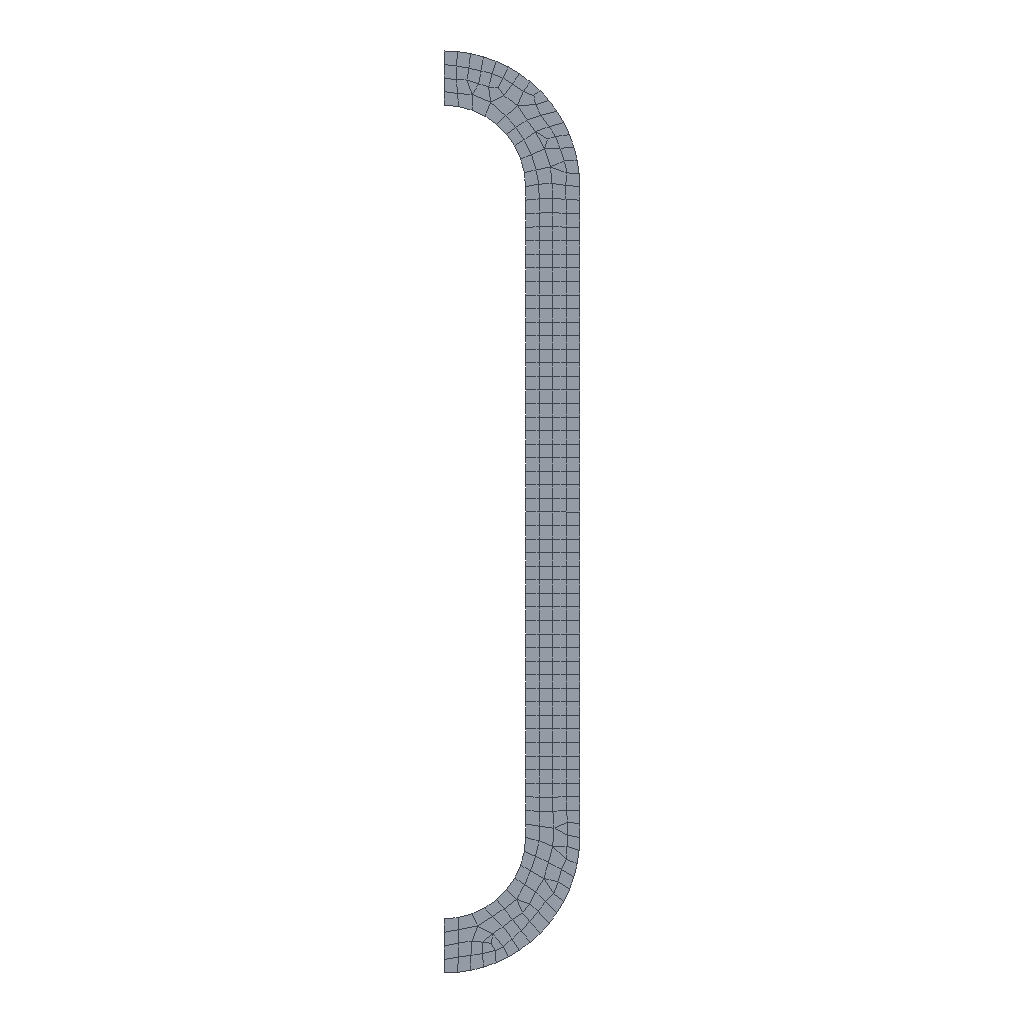Simulation study | ansys workbench
Set-up summary:
category,name,step,type,value,unit,region
solver,ansys_workbench
units,mm-N-s-tonne (MPa),,stated,"/units,MPA"
analysis,LS1,,static
load_step,LS1,LS1,static,nsubst=1; time=1
mesh,nodes,,,1039
mesh,elements,,,371
element_type,PLANE183,,,297
element_type,SURF153,,,66
element_type,CONTA172,,,8
material,?,,E,210000,tonne s^-2 mm^-1
material,?,,nu,0.3
material,?,,density,7.85e-09,tonne mm^-3
load,Define Pressure Using Surface Effect Elements,LS1,pressure,150,,SURF153 #4
bc,,LS1,fixed,"[dofs=UX,UY n=2]",,node list
contact,contact 1,,bonded (always),element=CONTA172
named_set,REMOTEDISPALL,,node,1
Ansys APDL input file, long lists of numbers shortened:
/batch
/config,noeldb,1     ! force off writing results to database
*get,_wallstrt,active,,time,wall
! ANSYS input file written by Workbench version 2021 R1
! File used for geometry attach:
/title,________--____ (A5)
! ****** Begin Custom Load Command Snippet ******
/COM, ACT Extensions:
/COM,     LSDYNA, 2021.1
/COM,
! ****** End   Custom Load Command Snippet ******
*DIM,_wb_ProjectScratch_dir,string,248
_wb_ProjectScratch_dir(1) = ''
*DIM,_wb_SolverFiles_dir,string,248
_wb_SolverFiles_dir(1) = ''
*DIM,_wb_userfiles_dir,string,248
_wb_userfiles_dir(1) = ''
/com,--- Data in consistent NMM units. See Solving Units in the help system for more information.
/units,MPA
/nopr
/wb,file,start              !  signify a WB generated input file
/prep7
! Turn off shape checking because checks already performed inside WB mesher.
! See help system for more information.
SHPP,OFF,,NOWARN
/nolist
etcon,set             ! allow ANSYS to choose best KEYOP's for 180x elements, resets any applicable keyopt to MAPDL defaults
/com,*********** Nodes for the whole assembly ***********
nblock,3,,1141
(1i9,3e20.9e3)
        1     0.000000000E+00     0.000000000E+00     0.000000000E+00
! (1037 more lines like these left out)
-1
/com,*********** Nodes for all Remote Points ***********
nblock,3
(1i9,3e20.9e3)
     1039     3.516693785E+01     1.699999993E+02     0.000000000E+00
-1
/wb,elem,start            !  set before creation of elements
/com,*********** Elements for Body 1 "______2-FreeParts|NONE" ***********
et,1,183
keyo,1,3,1
eblock,19,solid,,297
(19i9)
        1        1        1        1        0        0        0        0        8        0        1      158      197      195      195      688      826      195      687
! (296 more lines like these left out)
-1
/wb,elem,end               !  done creating elements
/com,*********** Send User Defined Coordinate System(s) ***********
csys,0
toffst,273.15,  ! Temperature offset from absolute zero
/com,*********** Set Reference Temperature ***********
tref,22.
/wb,mat,start              !  starting to send materials
/com,*********** Send Materials ***********
MP,DENS,1,7.85e-09,	! tonne mm^-3
MP,EX,1,210000,	! tonne s^-2 mm^-1
MP,NUXY,1,0.3,
/wb,mat,end                !  done sending materials
/com,*********** Send Sheet Properties ***********
!************************* Model Summary ********************
!______2-FreeParts|NONE,	合金钢,	matid,	1
!************************* End Model Summary ********************
! get the diagonal of the bounding box. Needed later for other things
*get,_xmin,node,,mnloc,x
*get,_ymin,node,,mnloc,y
*get,_zmin,node,,mnloc,z
*get,_xmax,node,,mxloc,x
*get,_ymax,node,,mxloc,y
*get,_zmax,node,,mxloc,z
_ASMDIAG=(_xmax-_xmin)*(_xmax-_xmin)+(_ymax-_ymin)*(_ymax-_ymin)+(_zmax-_zmin)*(_zmax-_zmin)
_ASMDIAG=SQRT(_ASMDIAG)
/wb,contact,start          !  starting to send contact
/wb,contact,end            !  done creating contacts
/golist
/wb,load,start             !  starting to send loads
/com,*********** Create Remote Point "内部远程点" ***********
! -------- Remote Point Used by "远程位移" --------
*set,tid,3
*set,cid,2
et,cid,172
et,tid,169
keyo,tid,2,1               ! Don't fix the pilot node
keyo,tid,4,000111
keyo,cid,12,5              ! Bonded Contact
keyo,cid,4,1               ! Deformable RBE3 style load
keyo,cid,2,2               ! MPC style contact
eblock,10,,,8
(15i9)
      299        2        2        2        0       84       85      537
! (7 more lines like these left out)
-1
*set,_npilot,1039
_npilot71=_npilot
type,tid
mat ,cid
real,cid
tshape,pilo
en,307,_npilot
tshape
/com,*********** Define Pressure Using Surface Effect Elements ***********
et,4,153
keyop,4,3,10        ! get plane stress option and thickness from underlying element
eblock,10,,,66
(15i9)
      308        4        4        4        0      143      151      654
! (65 more lines like these left out)
-1
esel,s,type,,4
keyop,4,7,0                ! Use deformed area for application of load
esel,all
/com,*********** Construct Remote Displacement ***********
/COM,*** Create a component for all remote displacements ***
CMBLOCK,REMOTEDISPALL,NODE,        1
(8i10)
      1039
esel,all
/com,*********** Define Rotational Velocity ***********
cglo,0.,170.,0.
/gst,on,on
fini
*get,_numnode,node,0,count
*get,_numelem,elem,0,count
*get, _MAXELEMNUM, elem, 0, NUM, MAX
*get, _MAXNODENUM, node, 0, NUM, MAX
*get, _MAXELEMTYPE, etyp, 0, NUM, MAX
*get, _MAXREALCONST, real, 0, NUM, MAX
/go
/wb,load,end               !  done creating loads
/com,--- Number of total nodes = %_numnode%
/com,--- Number of contact elements = 74
/com,--- Number of spring elements = 0
/com,--- Number of bearing elements = 0
/com,--- Number of solid elements = 297
/com,--- Number of condensed parts = 0
/com,--- Number of total elements = %_numelem%
*get,_wallbsol,active,,time,wall
/com,****************************************************************************
/com,*************************    SOLUTION       ********************************
/com,****************************************************************************
/solu
antype,0                   ! static analysis
_thickRatio=  0     ! Ratio of thick parts in the model
eqsl,sparse,,,,,1
cntr,print,1               ! print out contact info and also make no initial contact an error
dmpoption,emat,no             ! Don't combine emat file for DANSYS
dmpoption,esav,no             ! Don't combine esav file for DANSYS
nldiag,cont,iter           ! print out contact info each equilibrium iteration
rescontrol,,none                 ! Do not keep any restart files
/com,****************************************************
/com,******************* SOLVE FOR LS 1 OF 1 ****************
esel,s,type,,4
nsle
sf,all,pres,150.
nsel,all
esel,all
d,1039,ux,0.
d,1039,uy,0.
cgom,0.0,586.431
esel,all
/nopr
/gopr
/nolist
nsub,1,1,1
time,1.
outres,erase
outres,all,none
outres,nsol,all,
outres,rsol,all
outres,eangl,all
outres,etmp,all
outres,veng,all
outres,strs,all,
outres,epel,all,
outres,eppl,all,
outres,cont,all,
! *********** WB SOLVE COMMAND ***********
! check interactive state
*get,ANSINTER_,active,,int
*if,ANSINTER_,ne,0,then
/eof
*endif
solve
/com *************** Write FE CONNECTORS *********
CEWRITE,file,ce,,INTE
/com,****************************************************
/com,*************** FINISHED SOLVE FOR LS 1 *************
*get,_wallasol,active,,time,wall
/nopr
*get,_numnode,node,0,count
*get,_numelem,elem,0,count
*get, _MAXELEMNUM, elem, 0, NUM, MAX
*get, _MAXNODENUM, node, 0, NUM, MAX,,,INTERNAL
*get, _MAXELEMTYPE, etyp, 0, NUM, MAX
*get, _MAXREALCONST, real, 0, NUM, MAX
/gopr
/post1
xmlo,ENCODING,ISO-8859-1
xmlo,parm
/xml,parm,xml
fini
/gopr
*get,_walldone,active,,time,wall
_preptime=(_wallbsol-_wallstrt)*3600
_solvtime=(_wallasol-_wallbsol)*3600
_posttime=(_walldone-_wallasol)*3600
_totaltim=(_walldone-_wallstrt)*3600
*get,_dlbratio,active,0,solu,dlbr
*get,_combtime,active,0,solu,comb
/com,--- Total number of nodes = %_numnode%
/com,--- Total number of elements = %_numelem%
/com,--- Element load balance ratio = %_dlbratio%
/com,--- Time to combine distributed files = %_combtime%
/wb,file,end               ! done with WB generated input
Results summary:
result,analyses[0].index,,,1
result,analyses[0].system,,,SYS
result,analyses[0].deck,,,deck.dat
result,analyses[0].solve_status,,,completed
result,analyses[0].analysis_type,,,static
result,analyses[0].physics,,,mechanical
result,analyses[0].unit_system,,,"NMM: mm, ton, N, s, mV, mA, degC"
result,analyses[0].n_sets,,,1
result,analyses[0].load_steps[0].set,set=1,,1
result,analyses[0].load_steps[0].time_or_freq,set=1,,1
result,analyses[0].load_steps[0].max_displacement_magnitude,set=1,,0.05179
result,analyses[0].load_steps[0].max_von_mises_nodal,set=1,,409.289
result,analyses[0].load_steps[0].reaction_force_sum_xyz[1],set=1,,-18.291
result,analyses[0].load_steps[0].reaction_force_sum_xyz[2],set=1,,2.42164e-08
result,analyses[0].load_steps[0].reaction_force_sum_xyz[3],set=1,,0
result,geometry_export[0][0],,,.step
result,geometry_export[0][1],,,ok
result,geometry_export[0][2],,,1